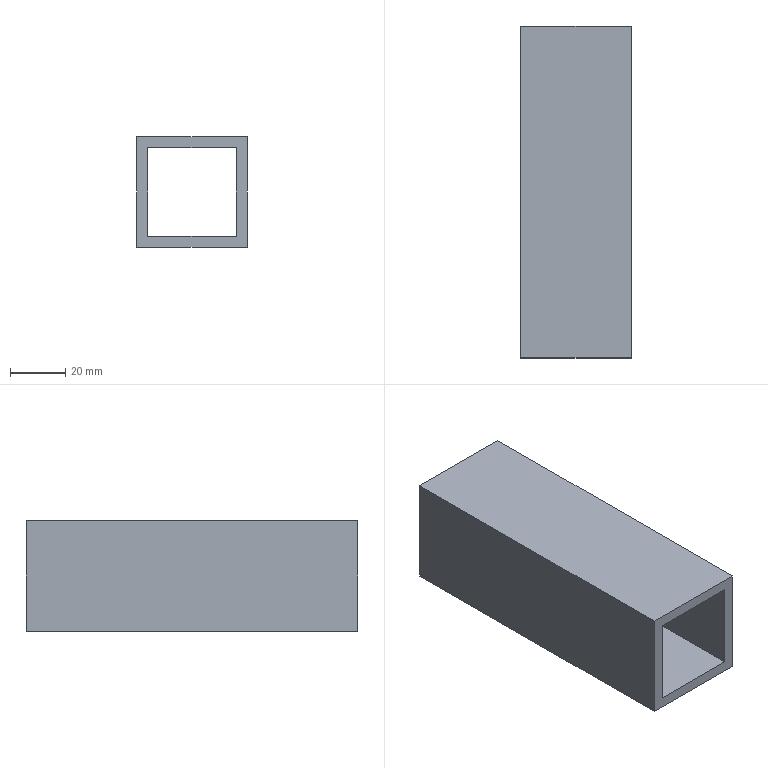Part | NX | features solid 2 | 1 solid | 10 faces | box 40 x 120 x 40 mm | volume 69120 mm3 | plane 10
STEP:
#1=CARTESIAN_POINT('',(695.,-180.,-45.));
#2=VERTEX_POINT('',#1);
#3=CARTESIAN_POINT('',(695.,-180.,-85.));
#4=VERTEX_POINT('',#3);
#5=CARTESIAN_POINT('',(695.,-180.,-40.));
#6=DIRECTION('',(0.,0.,-1.));
#7=VECTOR('',#6,1000.);
#8=LINE('',#5,#7);
#9=EDGE_CURVE('',#2,#4,#8,.T.);
#10=ORIENTED_EDGE('',*,*,#9,.T.);
#11=CARTESIAN_POINT('',(695.,-60.,-85.));
#12=VERTEX_POINT('',#11);
#13=CARTESIAN_POINT('',(695.,1714.393,-85.));
#14=DIRECTION('',(0.,1.,0.));
#15=VECTOR('',#14,1000.);
#16=LINE('',#13,#15);
#17=EDGE_CURVE('',#4,#12,#16,.T.);
#18=ORIENTED_EDGE('',*,*,#17,.T.);
#19=CARTESIAN_POINT('',(695.,-60.,-45.));
#20=VERTEX_POINT('',#19);
#21=CARTESIAN_POINT('',(695.,-60.,-40.));
#22=DIRECTION('',(0.,0.,1.));
#23=VECTOR('',#22,1000.);
#24=LINE('',#21,#23);
#25=EDGE_CURVE('',#12,#20,#24,.T.);
#26=ORIENTED_EDGE('',*,*,#25,.T.);
#27=CARTESIAN_POINT('',(695.,1714.393,-45.));
#28=DIRECTION('',(0.,-1.,0.));
#29=VECTOR('',#28,1000.);
#30=LINE('',#27,#29);
#31=EDGE_CURVE('',#20,#2,#30,.T.);
#32=ORIENTED_EDGE('',*,*,#31,.T.);
#33=EDGE_LOOP('',(#10,#18,#26,#32));
#34=FACE_BOUND('',#33,.T.);
#35=CARTESIAN_POINT('',(695.,1629.393,-40.));
#36=DIRECTION('',(-1.,0.,0.));
#37=DIRECTION('',(0.,0.,-1.));
#38=AXIS2_PLACEMENT_3D('',#35,#36,#37);
#39=PLANE('',#38);
#40=ADVANCED_FACE('',(#34),#39,.F.);
#41=CARTESIAN_POINT('',(655.,-180.,-45.));
#42=VERTEX_POINT('',#41);
#43=CARTESIAN_POINT('',(35.,-180.,-45.));
#44=DIRECTION('',(1.,0.,0.));
#45=VECTOR('',#44,1000.);
#46=LINE('',#43,#45);
#47=EDGE_CURVE('',#42,#2,#46,.T.);
#48=ORIENTED_EDGE('',*,*,#47,.T.);
#49=ORIENTED_EDGE('',*,*,#31,.F.);
#50=CARTESIAN_POINT('',(655.,-60.,-45.));
#51=VERTEX_POINT('',#50);
#52=CARTESIAN_POINT('',(35.,-60.,-45.));
#53=DIRECTION('',(-1.,0.,0.));
#54=VECTOR('',#53,1000.);
#55=LINE('',#52,#54);
#56=EDGE_CURVE('',#20,#51,#55,.T.);
#57=ORIENTED_EDGE('',*,*,#56,.T.);
#58=CARTESIAN_POINT('',(655.,1714.393,-45.));
#59=DIRECTION('',(0.,1.,0.));
#60=VECTOR('',#59,1000.);
#61=LINE('',#58,#60);
#62=EDGE_CURVE('',#42,#51,#61,.T.);
#63=ORIENTED_EDGE('',*,*,#62,.F.);
#64=EDGE_LOOP('',(#48,#49,#57,#63));
#65=FACE_BOUND('',#64,.T.);
#66=CARTESIAN_POINT('',(35.,1714.393,-45.));
#67=DIRECTION('',(0.,0.,-1.));
#68=DIRECTION('',(1.,0.,0.));
#69=AXIS2_PLACEMENT_3D('',#66,#67,#68);
#70=PLANE('',#69);
#71=ADVANCED_FACE('',(#65),#70,.F.);
#72=CARTESIAN_POINT('',(655.,-180.,-85.));
#73=VERTEX_POINT('',#72);
#74=CARTESIAN_POINT('',(75.,-180.,-85.));
#75=DIRECTION('',(-1.,0.,0.));
#76=VECTOR('',#75,1000.);
#77=LINE('',#74,#76);
#78=EDGE_CURVE('',#4,#73,#77,.T.);
#79=ORIENTED_EDGE('',*,*,#78,.T.);
#80=CARTESIAN_POINT('',(655.,-60.,-85.));
#81=VERTEX_POINT('',#80);
#82=CARTESIAN_POINT('',(655.,1629.393,-85.));
#83=DIRECTION('',(0.,1.,0.));
#84=VECTOR('',#83,1000.);
#85=LINE('',#82,#84);
#86=EDGE_CURVE('',#73,#81,#85,.T.);
#87=ORIENTED_EDGE('',*,*,#86,.T.);
#88=CARTESIAN_POINT('',(75.,-60.,-85.));
#89=DIRECTION('',(1.,0.,0.));
#90=VECTOR('',#89,1000.);
#91=LINE('',#88,#90);
#92=EDGE_CURVE('',#81,#12,#91,.T.);
#93=ORIENTED_EDGE('',*,*,#92,.T.);
#94=ORIENTED_EDGE('',*,*,#17,.F.);
#95=EDGE_LOOP('',(#79,#87,#93,#94));
#96=FACE_BOUND('',#95,.T.);
#97=CARTESIAN_POINT('',(75.,1714.393,-85.));
#98=DIRECTION('',(0.,0.,1.));
#99=DIRECTION('',(-1.,0.,0.));
#100=AXIS2_PLACEMENT_3D('',#97,#98,#99);
#101=PLANE('',#100);
#102=ADVANCED_FACE('',(#96),#101,.F.);
#103=CARTESIAN_POINT('',(655.,-180.,-70.));
#104=DIRECTION('',(0.,0.,1.));
#105=VECTOR('',#104,1000.);
#106=LINE('',#103,#105);
#107=EDGE_CURVE('',#73,#42,#106,.T.);
#108=ORIENTED_EDGE('',*,*,#107,.T.);
#109=ORIENTED_EDGE('',*,*,#62,.T.);
#110=CARTESIAN_POINT('',(655.,-60.,-70.));
#111=DIRECTION('',(0.,0.,-1.));
#112=VECTOR('',#111,1000.);
#113=LINE('',#110,#112);
#114=EDGE_CURVE('',#51,#81,#113,.T.);
#115=ORIENTED_EDGE('',*,*,#114,.T.);
#116=ORIENTED_EDGE('',*,*,#86,.F.);
#117=EDGE_LOOP('',(#108,#109,#115,#116));
#118=FACE_BOUND('',#117,.T.);
#119=CARTESIAN_POINT('',(655.,1629.393,-70.));
#120=DIRECTION('',(1.,0.,0.));
#121=DIRECTION('',(0.,0.,1.));
#122=AXIS2_PLACEMENT_3D('',#119,#120,#121);
#123=PLANE('',#122);
#124=ADVANCED_FACE('',(#118),#123,.F.);
#125=CARTESIAN_POINT('',(691.,-60.,-81.));
#126=VERTEX_POINT('',#125);
#127=CARTESIAN_POINT('',(691.,-60.,-49.));
#128=VERTEX_POINT('',#127);
#129=CARTESIAN_POINT('',(691.,-60.,-40.));
#130=DIRECTION('',(0.,0.,1.));
#131=VECTOR('',#130,1000.);
#132=LINE('',#129,#131);
#133=EDGE_CURVE('',#126,#128,#132,.T.);
#134=ORIENTED_EDGE('',*,*,#133,.T.);
#135=CARTESIAN_POINT('',(659.,-60.,-49.));
#136=VERTEX_POINT('',#135);
#137=CARTESIAN_POINT('',(35.,-60.,-49.));
#138=DIRECTION('',(-1.,0.,0.));
#139=VECTOR('',#138,1000.);
#140=LINE('',#137,#139);
#141=EDGE_CURVE('',#128,#136,#140,.T.);
#142=ORIENTED_EDGE('',*,*,#141,.T.);
#143=CARTESIAN_POINT('',(659.,-60.,-81.));
#144=VERTEX_POINT('',#143);
#145=CARTESIAN_POINT('',(659.,-60.,-70.));
#146=DIRECTION('',(0.,0.,-1.));
#147=VECTOR('',#146,1000.);
#148=LINE('',#145,#147);
#149=EDGE_CURVE('',#136,#144,#148,.T.);
#150=ORIENTED_EDGE('',*,*,#149,.T.);
#151=CARTESIAN_POINT('',(75.,-60.,-81.));
#152=DIRECTION('',(1.,0.,0.));
#153=VECTOR('',#152,1000.);
#154=LINE('',#151,#153);
#155=EDGE_CURVE('',#144,#126,#154,.T.);
#156=ORIENTED_EDGE('',*,*,#155,.T.);
#157=EDGE_LOOP('',(#134,#142,#150,#156));
#158=FACE_BOUND('',#157,.T.);
#159=ORIENTED_EDGE('',*,*,#92,.F.);
#160=ORIENTED_EDGE('',*,*,#114,.F.);
#161=ORIENTED_EDGE('',*,*,#56,.F.);
#162=ORIENTED_EDGE('',*,*,#25,.F.);
#163=EDGE_LOOP('',(#159,#160,#161,#162));
#164=FACE_BOUND('',#163,.T.);
#165=CARTESIAN_POINT('',(695.,-60.,-45.));
#166=DIRECTION('',(0.,1.,0.));
#167=DIRECTION('',(0.,0.,1.));
#168=AXIS2_PLACEMENT_3D('',#165,#166,#167);
#169=PLANE('',#168);
#170=ADVANCED_FACE('',(#158,#164),#169,.T.);
#171=CARTESIAN_POINT('',(691.,-180.,-49.));
#172=VERTEX_POINT('',#171);
#173=CARTESIAN_POINT('',(691.,1714.393,-49.));
#174=DIRECTION('',(0.,-1.,0.));
#175=VECTOR('',#174,1000.);
#176=LINE('',#173,#175);
#177=EDGE_CURVE('',#128,#172,#176,.T.);
#178=ORIENTED_EDGE('',*,*,#177,.F.);
#179=ORIENTED_EDGE('',*,*,#133,.F.);
#180=CARTESIAN_POINT('',(691.,-180.,-81.));
#181=VERTEX_POINT('',#180);
#182=CARTESIAN_POINT('',(691.,1714.393,-81.));
#183=DIRECTION('',(0.,1.,0.));
#184=VECTOR('',#183,1000.);
#185=LINE('',#182,#184);
#186=EDGE_CURVE('',#181,#126,#185,.T.);
#187=ORIENTED_EDGE('',*,*,#186,.F.);
#188=CARTESIAN_POINT('',(691.,-180.,-40.));
#189=DIRECTION('',(0.,0.,-1.));
#190=VECTOR('',#189,1000.);
#191=LINE('',#188,#190);
#192=EDGE_CURVE('',#172,#181,#191,.T.);
#193=ORIENTED_EDGE('',*,*,#192,.F.);
#194=EDGE_LOOP('',(#178,#179,#187,#193));
#195=FACE_BOUND('',#194,.T.);
#196=CARTESIAN_POINT('',(691.,1629.393,-40.));
#197=DIRECTION('',(-1.,0.,0.));
#198=DIRECTION('',(0.,0.,-1.));
#199=AXIS2_PLACEMENT_3D('',#196,#197,#198);
#200=PLANE('',#199);
#201=ADVANCED_FACE('',(#195),#200,.T.);
#202=CARTESIAN_POINT('',(659.,-180.,-49.));
#203=VERTEX_POINT('',#202);
#204=CARTESIAN_POINT('',(659.,1714.393,-49.));
#205=DIRECTION('',(0.,1.,0.));
#206=VECTOR('',#205,1000.);
#207=LINE('',#204,#206);
#208=EDGE_CURVE('',#203,#136,#207,.T.);
#209=ORIENTED_EDGE('',*,*,#208,.T.);
#210=ORIENTED_EDGE('',*,*,#141,.F.);
#211=ORIENTED_EDGE('',*,*,#177,.T.);
#212=CARTESIAN_POINT('',(35.,-180.,-49.));
#213=DIRECTION('',(1.,0.,0.));
#214=VECTOR('',#213,1000.);
#215=LINE('',#212,#214);
#216=EDGE_CURVE('',#203,#172,#215,.T.);
#217=ORIENTED_EDGE('',*,*,#216,.F.);
#218=EDGE_LOOP('',(#209,#210,#211,#217));
#219=FACE_BOUND('',#218,.T.);
#220=CARTESIAN_POINT('',(35.,1714.393,-49.));
#221=DIRECTION('',(0.,0.,-1.));
#222=DIRECTION('',(1.,0.,0.));
#223=AXIS2_PLACEMENT_3D('',#220,#221,#222);
#224=PLANE('',#223);
#225=ADVANCED_FACE('',(#219),#224,.T.);
#226=ORIENTED_EDGE('',*,*,#186,.T.);
#227=ORIENTED_EDGE('',*,*,#155,.F.);
#228=CARTESIAN_POINT('',(659.,-180.,-81.));
#229=VERTEX_POINT('',#228);
#230=CARTESIAN_POINT('',(659.,1629.393,-81.));
#231=DIRECTION('',(0.,1.,0.));
#232=VECTOR('',#231,1000.);
#233=LINE('',#230,#232);
#234=EDGE_CURVE('',#229,#144,#233,.T.);
#235=ORIENTED_EDGE('',*,*,#234,.F.);
#236=CARTESIAN_POINT('',(75.,-180.,-81.));
#237=DIRECTION('',(-1.,0.,0.));
#238=VECTOR('',#237,1000.);
#239=LINE('',#236,#238);
#240=EDGE_CURVE('',#181,#229,#239,.T.);
#241=ORIENTED_EDGE('',*,*,#240,.F.);
#242=EDGE_LOOP('',(#226,#227,#235,#241));
#243=FACE_BOUND('',#242,.T.);
#244=CARTESIAN_POINT('',(75.,1714.393,-81.));
#245=DIRECTION('',(0.,0.,1.));
#246=DIRECTION('',(-1.,0.,0.));
#247=AXIS2_PLACEMENT_3D('',#244,#245,#246);
#248=PLANE('',#247);
#249=ADVANCED_FACE('',(#243),#248,.T.);
#250=ORIENTED_EDGE('',*,*,#234,.T.);
#251=ORIENTED_EDGE('',*,*,#149,.F.);
#252=ORIENTED_EDGE('',*,*,#208,.F.);
#253=CARTESIAN_POINT('',(659.,-180.,-70.));
#254=DIRECTION('',(0.,0.,1.));
#255=VECTOR('',#254,1000.);
#256=LINE('',#253,#255);
#257=EDGE_CURVE('',#229,#203,#256,.T.);
#258=ORIENTED_EDGE('',*,*,#257,.F.);
#259=EDGE_LOOP('',(#250,#251,#252,#258));
#260=FACE_BOUND('',#259,.T.);
#261=CARTESIAN_POINT('',(659.,1629.393,-70.));
#262=DIRECTION('',(1.,0.,0.));
#263=DIRECTION('',(0.,0.,1.));
#264=AXIS2_PLACEMENT_3D('',#261,#262,#263);
#265=PLANE('',#264);
#266=ADVANCED_FACE('',(#260),#265,.T.);
#267=ORIENTED_EDGE('',*,*,#257,.T.);
#268=ORIENTED_EDGE('',*,*,#216,.T.);
#269=ORIENTED_EDGE('',*,*,#192,.T.);
#270=ORIENTED_EDGE('',*,*,#240,.T.);
#271=EDGE_LOOP('',(#267,#268,#269,#270));
#272=FACE_BOUND('',#271,.T.);
#273=ORIENTED_EDGE('',*,*,#78,.F.);
#274=ORIENTED_EDGE('',*,*,#9,.F.);
#275=ORIENTED_EDGE('',*,*,#47,.F.);
#276=ORIENTED_EDGE('',*,*,#107,.F.);
#277=EDGE_LOOP('',(#273,#274,#275,#276));
#278=FACE_BOUND('',#277,.T.);
#279=CARTESIAN_POINT('',(655.,-180.,-45.));
#280=DIRECTION('',(0.,-1.,0.));
#281=DIRECTION('',(0.,0.,-1.));
#282=AXIS2_PLACEMENT_3D('',#279,#280,#281);
#283=PLANE('',#282);
#284=ADVANCED_FACE('',(#272,#278),#283,.T.);
#285=CLOSED_SHELL('',(#40,#71,#102,#124,#170,#201,#225,#249,#266,#284));
#286=MANIFOLD_SOLID_BREP('',#285);
#287=(LENGTH_UNIT()NAMED_UNIT(*)SI_UNIT(.MILLI.,.METRE.));
#288=UNCERTAINTY_MEASURE_WITH_UNIT(LENGTH_MEASURE(0.00001),#287,'','');
#289=(NAMED_UNIT(*)PLANE_ANGLE_UNIT()SI_UNIT($,.RADIAN.));
#290=(NAMED_UNIT(*)SI_UNIT($,.STERADIAN.)SOLID_ANGLE_UNIT());
#291=(GEOMETRIC_REPRESENTATION_CONTEXT(3)GLOBAL_UNCERTAINTY_ASSIGNED_CONTEXT((#288))GLOBAL_UNIT_ASSIGNED_CONTEXT((#287,#289,#290))REPRESENTATION_CONTEXT('',''));
#292=ADVANCED_BREP_SHAPE_REPRESENTATION('',(#286),#291);